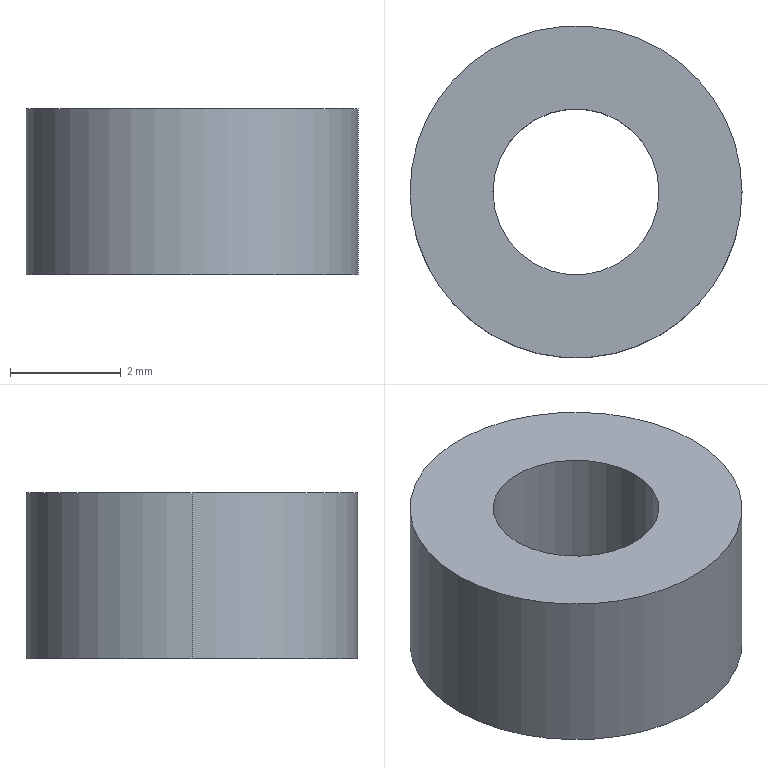Part | SolidWorks | features BaseBody 1 | 1 solid | 6 faces | box 6 x 6 x 3 mm | volume 63.617 mm3 | cylinder 4 | plane 2 | commonest cylinder face diameters 3 x2 6 x2
STEP:
#1=CARTESIAN_POINT('',(-114.97,214.3,173.));
#2=VERTEX_POINT('',#1);
#3=CARTESIAN_POINT('',(-117.97,214.3,173.));
#4=VERTEX_POINT('',#3);
#5=CARTESIAN_POINT('',(-116.47,214.3,173.));
#6=DIRECTION('',(0.,0.,-1.));
#7=DIRECTION('',(0.,-1.,0.));
#8=AXIS2_PLACEMENT_3D('',#5,#6,#7);
#9=CIRCLE('',#8,1.5);
#10=EDGE_CURVE('',#2,#4,#9,.T.);
#11=ORIENTED_EDGE('',*,*,#10,.T.);
#12=CARTESIAN_POINT('',(-117.97,214.3,176.));
#13=VERTEX_POINT('',#12);
#14=CARTESIAN_POINT('',(-117.97,214.3,173.));
#15=DIRECTION('',(0.,0.,1.));
#16=VECTOR('',#15,1000.);
#17=LINE('',#14,#16);
#18=EDGE_CURVE('',#4,#13,#17,.T.);
#19=ORIENTED_EDGE('',*,*,#18,.T.);
#20=CARTESIAN_POINT('',(-114.97,214.3,176.));
#21=VERTEX_POINT('',#20);
#22=CARTESIAN_POINT('',(-116.47,214.3,176.));
#23=DIRECTION('',(0.,0.,-1.));
#24=DIRECTION('',(0.,-1.,0.));
#25=AXIS2_PLACEMENT_3D('',#22,#23,#24);
#26=CIRCLE('',#25,1.5);
#27=EDGE_CURVE('',#21,#13,#26,.T.);
#28=ORIENTED_EDGE('',*,*,#27,.F.);
#29=CARTESIAN_POINT('',(-114.97,214.3,173.));
#30=DIRECTION('',(0.,0.,1.));
#31=VECTOR('',#30,1000.);
#32=LINE('',#29,#31);
#33=EDGE_CURVE('',#2,#21,#32,.T.);
#34=ORIENTED_EDGE('',*,*,#33,.F.);
#35=EDGE_LOOP('',(#11,#19,#28,#34));
#36=FACE_OUTER_BOUND('',#35,.T.);
#37=CARTESIAN_POINT('',(-116.47,214.3,173.));
#38=DIRECTION('',(0.,0.,1.));
#39=DIRECTION('',(1.,0.,0.));
#40=AXIS2_PLACEMENT_3D('',#37,#38,#39);
#41=CYLINDRICAL_SURFACE('',#40,1.5);
#42=ADVANCED_FACE('',(#36),#41,.F.);
#43=CARTESIAN_POINT('',(-119.47,214.3,173.));
#44=VERTEX_POINT('',#43);
#45=CARTESIAN_POINT('',(-113.47,214.3,173.));
#46=VERTEX_POINT('',#45);
#47=CARTESIAN_POINT('',(-116.47,214.3,173.));
#48=DIRECTION('',(0.,0.,-1.));
#49=DIRECTION('',(0.,-1.,0.));
#50=AXIS2_PLACEMENT_3D('',#47,#48,#49);
#51=CIRCLE('',#50,3.);
#52=EDGE_CURVE('',#44,#46,#51,.T.);
#53=ORIENTED_EDGE('',*,*,#52,.F.);
#54=CARTESIAN_POINT('',(-119.47,214.3,176.));
#55=VERTEX_POINT('',#54);
#56=CARTESIAN_POINT('',(-119.47,214.3,173.));
#57=DIRECTION('',(0.,0.,1.));
#58=VECTOR('',#57,1000.);
#59=LINE('',#56,#58);
#60=EDGE_CURVE('',#44,#55,#59,.T.);
#61=ORIENTED_EDGE('',*,*,#60,.T.);
#62=CARTESIAN_POINT('',(-113.47,214.3,176.));
#63=VERTEX_POINT('',#62);
#64=CARTESIAN_POINT('',(-116.47,214.3,176.));
#65=DIRECTION('',(0.,0.,-1.));
#66=DIRECTION('',(0.,-1.,0.));
#67=AXIS2_PLACEMENT_3D('',#64,#65,#66);
#68=CIRCLE('',#67,3.);
#69=EDGE_CURVE('',#55,#63,#68,.T.);
#70=ORIENTED_EDGE('',*,*,#69,.T.);
#71=CARTESIAN_POINT('',(-113.47,214.3,173.));
#72=DIRECTION('',(0.,0.,1.));
#73=VECTOR('',#72,1000.);
#74=LINE('',#71,#73);
#75=EDGE_CURVE('',#46,#63,#74,.T.);
#76=ORIENTED_EDGE('',*,*,#75,.F.);
#77=EDGE_LOOP('',(#53,#61,#70,#76));
#78=FACE_OUTER_BOUND('',#77,.T.);
#79=CARTESIAN_POINT('',(-116.47,214.3,173.));
#80=DIRECTION('',(0.,0.,1.));
#81=DIRECTION('',(1.,0.,0.));
#82=AXIS2_PLACEMENT_3D('',#79,#80,#81);
#83=CYLINDRICAL_SURFACE('',#82,3.);
#84=ADVANCED_FACE('',(#78),#83,.T.);
#85=ORIENTED_EDGE('',*,*,#60,.F.);
#86=CARTESIAN_POINT('',(-116.47,214.3,173.));
#87=DIRECTION('',(0.,0.,-1.));
#88=DIRECTION('',(0.,-1.,0.));
#89=AXIS2_PLACEMENT_3D('',#86,#87,#88);
#90=CIRCLE('',#89,3.);
#91=EDGE_CURVE('',#46,#44,#90,.T.);
#92=ORIENTED_EDGE('',*,*,#91,.F.);
#93=ORIENTED_EDGE('',*,*,#75,.T.);
#94=CARTESIAN_POINT('',(-116.47,214.3,176.));
#95=DIRECTION('',(0.,0.,-1.));
#96=DIRECTION('',(0.,-1.,0.));
#97=AXIS2_PLACEMENT_3D('',#94,#95,#96);
#98=CIRCLE('',#97,3.);
#99=EDGE_CURVE('',#63,#55,#98,.T.);
#100=ORIENTED_EDGE('',*,*,#99,.T.);
#101=EDGE_LOOP('',(#85,#92,#93,#100));
#102=FACE_OUTER_BOUND('',#101,.T.);
#103=CARTESIAN_POINT('',(-116.47,214.3,173.));
#104=DIRECTION('',(0.,0.,1.));
#105=DIRECTION('',(1.,0.,0.));
#106=AXIS2_PLACEMENT_3D('',#103,#104,#105);
#107=CYLINDRICAL_SURFACE('',#106,3.);
#108=ADVANCED_FACE('',(#102),#107,.T.);
#109=ORIENTED_EDGE('',*,*,#18,.F.);
#110=CARTESIAN_POINT('',(-116.47,214.3,173.));
#111=DIRECTION('',(0.,0.,-1.));
#112=DIRECTION('',(0.,-1.,0.));
#113=AXIS2_PLACEMENT_3D('',#110,#111,#112);
#114=CIRCLE('',#113,1.5);
#115=EDGE_CURVE('',#4,#2,#114,.T.);
#116=ORIENTED_EDGE('',*,*,#115,.T.);
#117=ORIENTED_EDGE('',*,*,#33,.T.);
#118=CARTESIAN_POINT('',(-116.47,214.3,176.));
#119=DIRECTION('',(0.,0.,-1.));
#120=DIRECTION('',(0.,-1.,0.));
#121=AXIS2_PLACEMENT_3D('',#118,#119,#120);
#122=CIRCLE('',#121,1.5);
#123=EDGE_CURVE('',#13,#21,#122,.T.);
#124=ORIENTED_EDGE('',*,*,#123,.F.);
#125=EDGE_LOOP('',(#109,#116,#117,#124));
#126=FACE_OUTER_BOUND('',#125,.T.);
#127=CARTESIAN_POINT('',(-116.47,214.3,173.));
#128=DIRECTION('',(0.,0.,1.));
#129=DIRECTION('',(1.,0.,0.));
#130=AXIS2_PLACEMENT_3D('',#127,#128,#129);
#131=CYLINDRICAL_SURFACE('',#130,1.5);
#132=ADVANCED_FACE('',(#126),#131,.F.);
#133=ORIENTED_EDGE('',*,*,#91,.T.);
#134=ORIENTED_EDGE('',*,*,#52,.T.);
#135=EDGE_LOOP('',(#133,#134));
#136=FACE_OUTER_BOUND('',#135,.T.);
#137=ORIENTED_EDGE('',*,*,#10,.F.);
#138=ORIENTED_EDGE('',*,*,#115,.F.);
#139=EDGE_LOOP('',(#137,#138));
#140=FACE_BOUND('',#139,.T.);
#141=CARTESIAN_POINT('',(-116.47,214.3,173.));
#142=DIRECTION('',(0.,0.,-1.));
#143=DIRECTION('',(-1.,0.,0.));
#144=AXIS2_PLACEMENT_3D('',#141,#142,#143);
#145=PLANE('',#144);
#146=ADVANCED_FACE('',(#136,#140),#145,.T.);
#147=ORIENTED_EDGE('',*,*,#99,.F.);
#148=ORIENTED_EDGE('',*,*,#69,.F.);
#149=EDGE_LOOP('',(#147,#148));
#150=FACE_OUTER_BOUND('',#149,.T.);
#151=ORIENTED_EDGE('',*,*,#27,.T.);
#152=ORIENTED_EDGE('',*,*,#123,.T.);
#153=EDGE_LOOP('',(#151,#152));
#154=FACE_BOUND('',#153,.T.);
#155=CARTESIAN_POINT('',(-116.47,214.3,176.));
#156=DIRECTION('',(0.,0.,-1.));
#157=DIRECTION('',(-1.,0.,0.));
#158=AXIS2_PLACEMENT_3D('',#155,#156,#157);
#159=PLANE('',#158);
#160=ADVANCED_FACE('',(#150,#154),#159,.F.);
#161=CLOSED_SHELL('',(#42,#84,#108,#132,#146,#160));
#162=MANIFOLD_SOLID_BREP('',#161);
#163=CARTESIAN_POINT('',(0.,0.,0.));
#164=DIRECTION('',(0.,0.,1.));
#165=DIRECTION('',(1.,0.,0.));
#166=AXIS2_PLACEMENT_3D('',#163,#164,#165);
#167=(LENGTH_UNIT()NAMED_UNIT(*)SI_UNIT(.MILLI.,.METRE.));
#168=UNCERTAINTY_MEASURE_WITH_UNIT(LENGTH_MEASURE(0.00001),#167,'','');
#169=(NAMED_UNIT(*)PLANE_ANGLE_UNIT()SI_UNIT($,.RADIAN.));
#170=(NAMED_UNIT(*)SI_UNIT($,.STERADIAN.)SOLID_ANGLE_UNIT());
#171=(GEOMETRIC_REPRESENTATION_CONTEXT(3)GLOBAL_UNCERTAINTY_ASSIGNED_CONTEXT((#168))GLOBAL_UNIT_ASSIGNED_CONTEXT((#167,#169,#170))REPRESENTATION_CONTEXT('',''));
#172=ADVANCED_BREP_SHAPE_REPRESENTATION('',(#162,#166),#171);